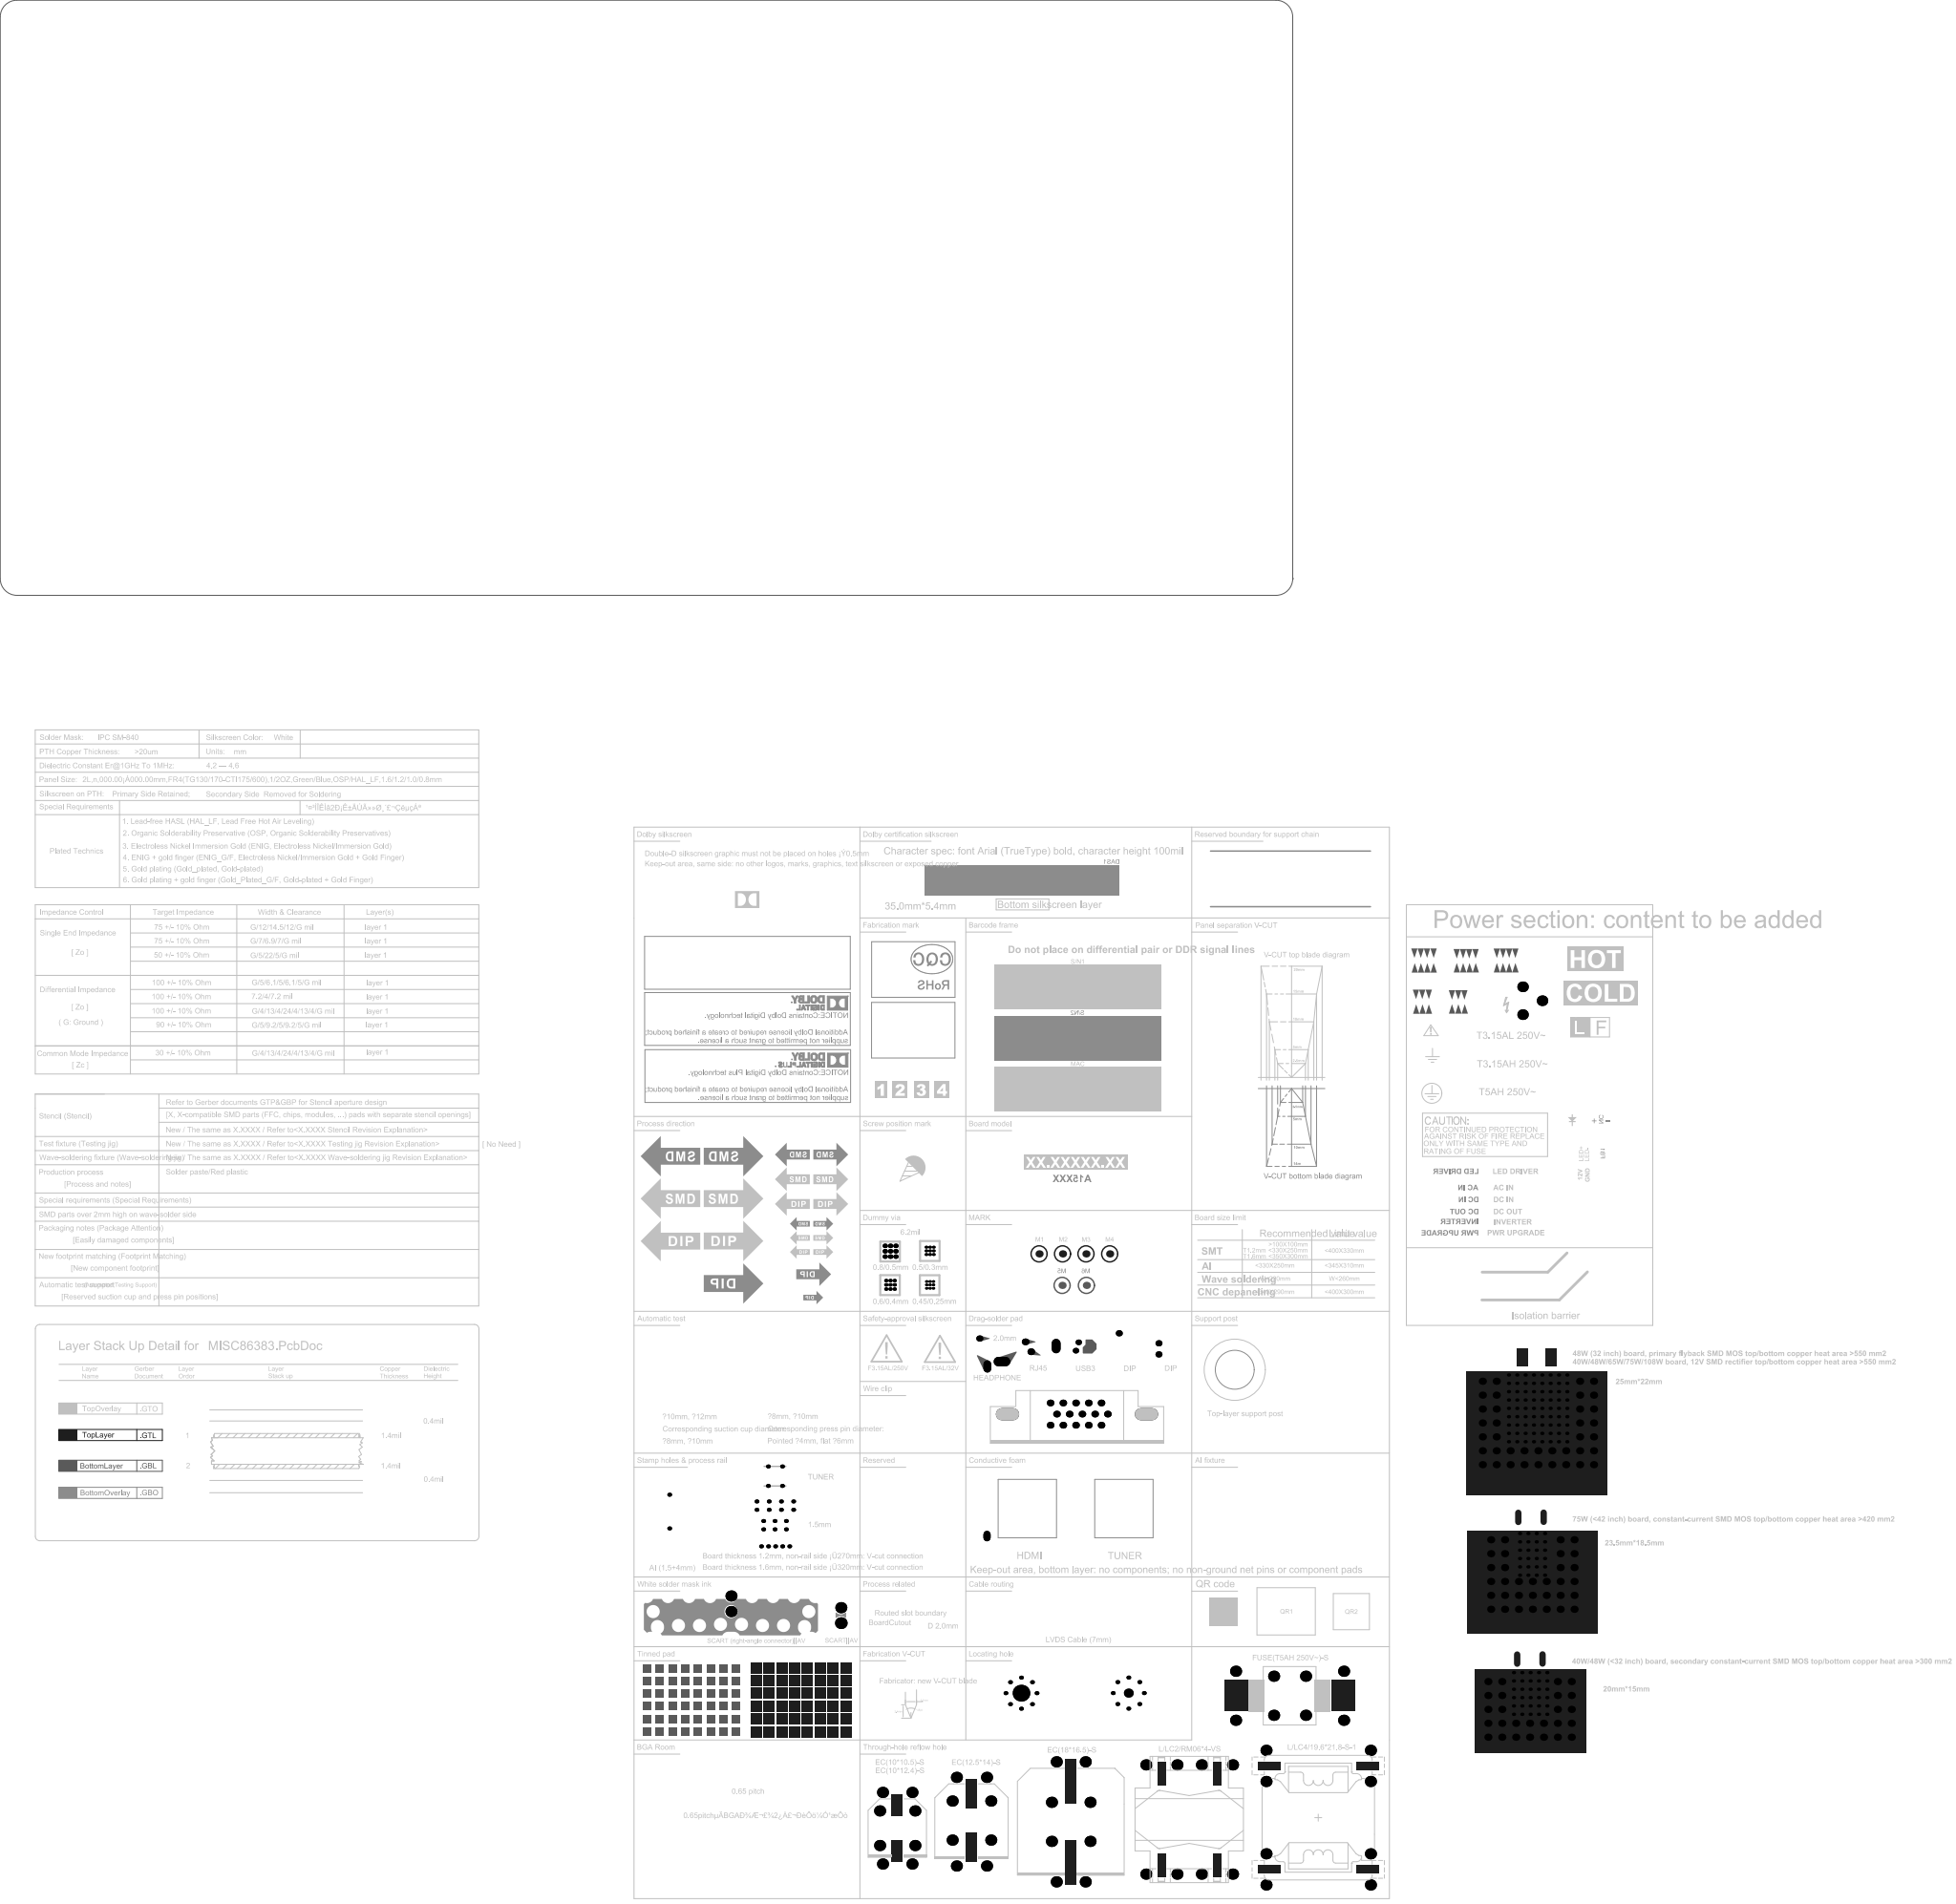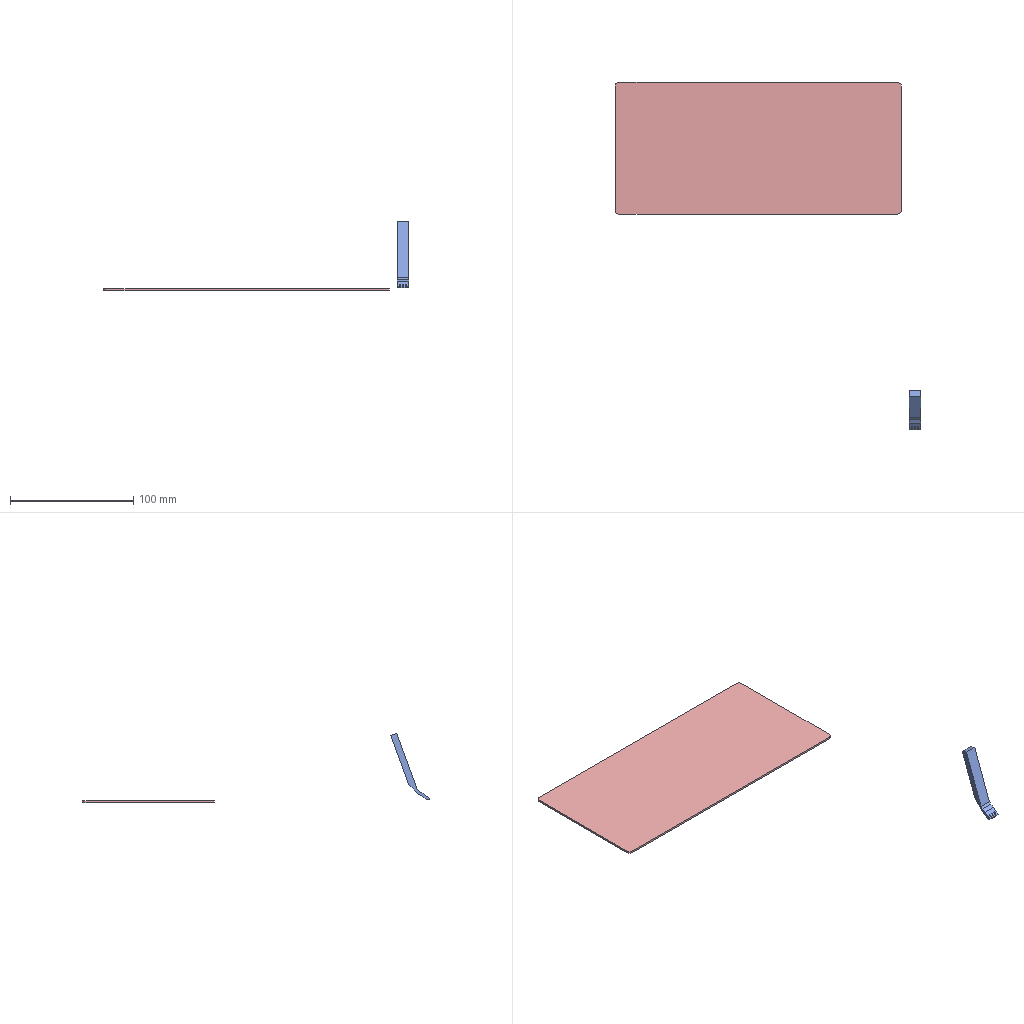Circuit board layout | Altium Designer | box 248.2 x 282.2 x 56.3 mm
Part placement:
Designator,Comment,Layer,Footprint,Center-X(mm),Center-Y(mm),Rotation
QR1,Comment,TopLayer,QRCODE-1,231.315,-182.683,0
QR2,Comment,TopLayer,QRCODE-2,243.05,-182.734,0
DBSR,NO DOLBY,BottomLayer,NO_DOLBY-SILK,-441.141,-338.525,180
M6,MARK,BottomLayer,MARK,195.385,-124.071,180
M5,MARK,BottomLayer,MARK,191.016,-124.071,180
XX.XXXXX.XX,PCB_NAME,TopLayer,PCB_NAME,188.493,-102.764,90
Manufacture_Info,Manufacture_Info,TopLayer,Manufacture_Info,164.258,-78.164,180
M4,MARK,TopLayer,MARK,199.576,-118.407,0
M3,MARK,TopLayer,MARK,195.309,-118.407,0
M2,MARK,TopLayer,MARK,191.092,-118.407,0
M1,MARK,TopLayer,MARK,186.876,-118.407,0
DBS0,DOLBY,BottomLayer,DOLBY-SILK,-441.141,-338.525,180
DBS7,DOLBY PLUS,BottomLayer,DOLBY_PLUS-SILK,-441.141,-338.525,180
CQC,CQC,TopLayer,CQC,-441.141,-338.525,360
A15XXX,PCB_TIME,TopLayer,PCB_TIME,195.63,-104.822,90
AI_V,Comment,TopLayer,AI_GRIPPER_V,243.535,-172.72,270
MAC,Comment,TopLayer,Barcode,193.802,-88.798,0
S/N2,Comment,BottomLayer,Barcode,193.802,-79.604,180
S/N1,Comment,TopLayer,Barcode,193.802,-70.409,0
DBS8,Comment,TopLayer,Double-D-SILK,-441.141,-338.525,0
DAS1,35.0*5.4mm,TopLayer,DOLBY_AS2,-441.141,-338.525,0